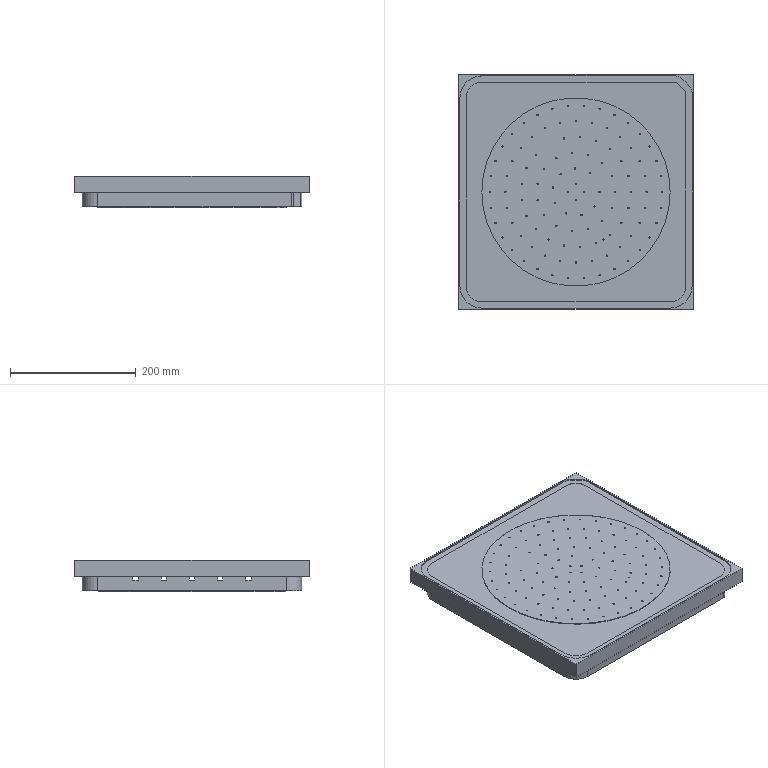NC program | NX | posted with a generic post | part box 374 x 374 x 49.5 mm
Lines 1180 to 2421 of 17720:
(03 , TOOL : D10)
N2352 M6
N2354 G53
N2356 G17 G0 G90 X-180. Y87.278 S7000 M3 M8
N2358 G43 Z105.5 H0
N2360 Z25.
N2362 G94 G1 Y125.441 Z23. F4000.
N2364 Y150.
N2366 G2 X-150. Y180. R30.
N2368 G1 X157.929
N2370 G2 X165. Y177.071 R10.
N2372 G1 X177.071 Y165.
N2374 G2 X180. Y157.929 R10.
N2376 G1 Y-150.
N2378 G2 X150. Y-180. R30.
N2380 G1 X-150.
N2382 G2 X-180. Y-150. R30.
N2384 G1 Y125.441
N2386 X-173.
N2388 Y150.
N2390 G2 X-150. Y173. R23.
N2392 G1 X157.929
N2394 G2 X160.05 Y172.121 R3.
N2396 G1 X172.121 Y160.05
N2398 G2 X173. Y157.929 R3.
N2400 G1 Y-150.
N2402 G2 X150. Y-173. R23.
N2404 G1 X-150.
N2406 G2 X-173. Y-150. R23.
N2408 G1 Y125.441
N2410 X-166.
N2412 Y150.
N2414 G2 X-150. Y166. R16.
N2416 G1 X156.272
N2418 X166. Y156.272
N2420 Y-150.
N2422 G2 X150. Y-166. R16.
N2424 G1 X-150.
N2426 G2 X-166. Y-150. R16.
N2428 G1 Y125.441
N2430 X-159.
N2432 Y150.
N2434 G2 X-150. Y159. R9.
N2436 G1 X153.373
N2438 X159. Y153.373
N2440 Y36.837
N2442 X152.
N2444 G3 X36.837 Y152. R156.4
N2446 G1 X30.515 Y153.705
N2448 X36.837 Y152.
N2450 X150.473
N2452 X152. Y150.473
N2454 Y75.33
N2456 X145.
N2458 G3 X75.33 Y145. R163.4
N2460 G1 X69.214 Y146.433
N2462 X75.33 Y145.
N2464 X145.
N2466 Y99.961
N2468 X138.
N2470 G3 X99.961 Y138. R170.4
N2472 G1 X94.665 Y139.672
N2474 X99.961 Y138.
N2476 X138.
N2478 Y119.623
N2480 X131.
N2482 G3 X119.623 Y131. R177.4
N2484 G1 X114.752 Y132.852
N2486 X119.623 Y131.
N2488 X131.
N2490 Y119.623
N2492 X132.852 Y114.752
N2494 X131. Y119.623
N2496 X138.
N2498 Y99.961
N2500 X139.672 Y94.665
N2502 X138. Y99.961
N2504 X145.
N2506 Y75.33
N2508 X146.433 Y69.214
N2510 X145. Y75.33
N2512 X152.
N2514 Y36.837
N2516 X153.705 Y30.515
N2518 X152. Y36.837
N2520 X159.
N2522 Y-150.
N2524 G2 X150. Y-159. R9.
N2526 G1 X36.837
N2528 Y-152.
N2530 G3 X152. Y-36.837 R156.4
N2532 G1 X153.705 Y-30.515
N2534 X152. Y-36.837
N2536 Y-150.
N2538 G2 X150. Y-152. R2.
N2540 G1 X75.33
N2542 Y-145.
N2544 G3 X145. Y-75.33 R163.4
N2546 G1 X146.433 Y-69.214
N2548 X145. Y-75.33
N2550 Y-145.
N2552 X99.961
N2554 Y-138.
N2556 G3 X138. Y-99.961 R170.4
N2558 G1 X139.672 Y-94.665
N2560 X138. Y-99.961
N2562 Y-138.
N2564 X119.623
N2566 Y-131.
N2568 G3 X131. Y-119.623 R177.4
N2570 G1 X132.852 Y-114.752
N2572 X131. Y-119.623
N2574 Y-131.
N2576 X119.623
N2578 X114.752 Y-132.852
N2580 X119.623 Y-131.
N2582 Y-138.
N2584 X99.961
N2586 X94.665 Y-139.672
N2588 X99.961 Y-138.
N2590 Y-145.
N2592 X75.33
N2594 X69.214 Y-146.433
N2596 X75.33 Y-145.
N2598 Y-152.
N2600 X36.837
N2602 X30.515 Y-153.705
N2604 X36.837 Y-152.
N2606 Y-159.
N2608 X-150.
N2610 G2 X-159. Y-150. R9.
N2612 G1 Y-36.837
N2614 X-152.
N2616 G3 X-36.837 Y-152. R156.4
N2618 G1 X-30.515 Y-153.705
N2620 X-36.837 Y-152.
N2622 X-150.
N2624 G2 X-152. Y-150. R2.
N2626 G1 Y-75.33
N2628 X-145.
N2630 G3 X-75.33 Y-145. R163.4
N2632 G1 X-69.214 Y-146.433
N2634 X-75.33 Y-145.
N2636 X-145.
N2638 Y-99.961
N2640 X-138.
N2642 G3 X-99.961 Y-138. R170.4
N2644 G1 X-94.665 Y-139.672
N2646 X-99.961 Y-138.
N2648 X-138.
N2650 Y-119.623
N2652 X-131.
N2654 G3 X-119.623 Y-131. R177.4
N2656 G1 X-114.752 Y-132.852
N2658 X-119.623 Y-131.
N2660 X-131.
N2662 Y-119.623
N2664 X-132.852 Y-114.752
N2666 X-131. Y-119.623
N2668 X-138.
N2670 Y-99.961
N2672 X-139.672 Y-94.665
N2674 X-138. Y-99.961
N2676 X-145.
N2678 Y-75.33
N2680 X-146.433 Y-69.214
N2682 X-145. Y-75.33
N2684 X-152.
N2686 Y-36.837
N2688 X-153.705 Y-30.515
N2690 X-152. Y-36.837
N2692 X-159.
N2694 Y125.441
N2696 X-152.
N2698 Y150.
N2700 G2 X-150. Y152. R2.
N2702 G1 X-36.837
N2704 X-30.515 Y153.705
N2706 X-36.837 Y152.
N2708 G3 X-152. Y36.837 R156.4
N2710 G1 X-153.705 Y30.515
N2712 X-152. Y36.837
N2714 X-150.639 Y36.507
N2716 G2 X36.507 Y150.639 R155.
N2718 X-150.639 Y36.507 R-155.
N2720 G1 X-152. Y36.837
N2722 Y125.441
N2724 X-145.
N2726 Y145.
N2728 X-75.33
N2730 X-69.214 Y146.433
N2732 X-75.33 Y145.
N2734 G3 X-145. Y75.33 R163.4
N2736 G1 X-146.433 Y69.214
N2738 X-145. Y75.33
N2740 Y125.441
N2742 X-138.
N2744 Y138.
N2746 X-99.961
N2748 X-94.665 Y139.672
N2750 X-99.961 Y138.
N2752 G3 X-138. Y99.961 R170.4
N2754 G1 X-139.672 Y94.665
N2756 X-138. Y99.961
N2758 Y125.441
N2760 X-131.
N2762 Y131.
N2764 X-119.623
N2766 X-114.752 Y132.852
N2768 X-119.623 Y131.
N2770 G3 X-131. Y119.623 R177.4
N2772 G1 X-132.852 Y114.752
N2774 X-131. Y119.623
N2776 Y125.441
N2778 G3 X-133. Y127.441 R2.
N2780 G1 Z24.
N2782 G0 Z105.5
N2784 X-148.274 Y-37.767
N2786 Z26.
N2788 G1 X-148.508 Y-36.927 Z25.954
N2790 X-150.341 Y-28.56 Z25.505
N2792 X-151.704 Y-20.104 Z25.057
N2794 X-152.591 Y-11.585 Z24.608
N2796 X-153. Y-3.03 Z24.159
N2798 Y0. Z24.
N2800 G2 X0. Y153. R153.
N2802 X-153. Y0. R-153.
N2804 G1 X-146.
N2806 G2 X0. Y146. R146.
N2808 X-146. Y0. R-146.
N2810 G1 X-139.
N2812 G2 X0. Y139. R139.
N2814 X-139. Y0. R-139.
N2816 G1 X-132.
N2818 G2 X0. Y132. R132.
N2820 X-132. Y0. R-132.
N2822 G1 X-125.
N2824 G2 X0. Y125. R125.
N2826 X-125. Y0. R-125.
N2828 G1 X-118.
N2830 G2 X0. Y118. R118.
N2832 X-118. Y0. R-118.
N2834 G1 X-111.
N2836 G2 X0. Y111. R111.
N2838 X-111. Y0. R-111.
N2840 G1 X-104.
N2842 G2 X0. Y104. R104.
N2844 X-104. Y0. R-104.
N2846 G1 X-97.
N2848 G2 X0. Y97. R97.
N2850 X-97. Y0. R-97.
N2852 G1 X-90.
N2854 G2 X0. Y90. R90.
N2856 X-90. Y0. R-90.
N2858 G1 X-83.
N2860 G2 X0. Y83. R83.
N2862 X-83. Y0. R-83.
N2864 G1 X-76.
N2866 G2 X0. Y76. R76.
N2868 X-76. Y0. R-76.
N2870 G1 X-69.
N2872 G2 X0. Y69. R69.
N2874 X-69. Y0. R-69.
N2876 G1 X-62.
N2878 G2 X0. Y62. R62.
N2880 X-62. Y0. R-62.
N2882 G1 X-55.
N2884 G2 X0. Y55. R55.
N2886 X-55. Y0. R-55.
N2888 G1 X-48.
N2890 G2 X0. Y48. R48.
N2892 X-48. Y0. R-48.
N2894 G1 X-41.
N2896 G2 X0. Y41. R41.
N2898 X-41. Y0. R-41.
N2900 G1 X-34.
N2902 G2 X0. Y34. R34.
N2904 X-34. Y0. R-34.
N2906 G1 X-27.
N2908 G2 X0. Y27. R27.
N2910 X-27. Y0. R-27.
N2912 G1 X-20.
N2914 G2 X0. Y20. R20.
N2916 X-20. Y0. R-20.
N2918 G1 X-13.
N2920 G2 X0. Y13. R13.
N2922 X-13. Y0. R-13.
N2924 G1 X-6.
N2926 G2 X0. Y6. R6.
N2928 X-6. Y0. R-6.
N2930 G1 X-1.5
N2932 G2 X0. Y1.5 R1.5
N2934 X-1.5 Y0. R-1.5
N2936 G3 X-3.5 Y2. R2.
N2938 G1 Z25.
N2940 G0 Z105.5
(003 , TOOL : D10)
N2942 X176.276 Y165.795
N2944 Z24.
N2946 G1 X177.619 Y164.452 Z23.998
N2948 X178.813 Y162.718 Z23.997
N2950 X179.618 Y160.774 Z23.995
N2952 X180. Y158.704 Z23.993
N2954 Y-151.342 Z23.722
N2956 X179.606 Y-155.026 Z23.719
N2958 X178.762 Y-158.633 Z23.716
N2960 X177.48 Y-162.109 Z23.713
N2962 X175.78 Y-165.401 Z23.709
N2964 X173.688 Y-168.458 Z23.706
N2966 X171.234 Y-171.234 Z23.703
N2968 X168.458 Y-173.688 Z23.7
N2970 X165.401 Y-175.78 Z23.696
N2972 X162.109 Y-177.48 Z23.693
N2974 X158.633 Y-178.762 Z23.69
N2976 X155.026 Y-179.606 Z23.687
N2978 X151.342 Y-180. Z23.683
N2980 X-151.342 Z23.419
N2982 X-155.026 Y-179.606 Z23.416
N2984 X-158.633 Y-178.762 Z23.413
N2986 X-162.109 Y-177.48 Z23.41
N2988 X-165.401 Y-175.78 Z23.406
N2990 X-168.458 Y-173.688 Z23.403
N2992 X-171.234 Y-171.234 Z23.4
N2994 X-173.688 Y-168.458 Z23.397
N2996 X-175.78 Y-165.401 Z23.393
N2998 X-177.48 Y-162.109 Z23.39
N3000 X-178.762 Y-158.633 Z23.387
N3002 X-179.606 Y-155.026 Z23.384
N3004 X-180. Y-151.342 Z23.381
N3006 Y151.342 Z23.116
N3008 X-179.606 Y155.026 Z23.113
N3010 X-178.762 Y158.633 Z23.11
N3012 X-177.48 Y162.109 Z23.107
N3014 X-175.78 Y165.401 Z23.103
N3016 X-173.688 Y168.458 Z23.1
N3018 X-171.234 Y171.234 Z23.097
N3020 X-168.458 Y173.688 Z23.094
N3022 X-165.401 Y175.78 Z23.091
N3024 X-162.109 Y177.48 Z23.087
N3026 X-158.633 Y178.762 Z23.084
N3028 X-155.026 Y179.606 Z23.081
N3030 X-151.342 Y180. Z23.078
N3032 X158.704 Z22.807
N3034 X160.774 Y179.618 Z22.805
N3036 X162.718 Y178.813 Z22.803
N3038 X164.452 Y177.619 Z22.802
N3040 X177.619 Y164.452 Z22.785
N3042 X178.813 Y162.718 Z22.783
N3044 X179.618 Y160.774 Z22.782
N3046 X180. Y158.704 Z22.78
N3048 Y-151.342 Z22.509
N3050 X179.606 Y-155.026 Z22.506
N3052 X178.762 Y-158.633 Z22.503
N3054 X177.48 Y-162.109 Z22.499
N3056 X175.78 Y-165.401 Z22.496
N3058 X173.688 Y-168.458 Z22.493
N3060 X171.234 Y-171.234 Z22.49
N3062 X168.458 Y-173.688 Z22.487
N3064 X165.401 Y-175.78 Z22.483
N3066 X162.109 Y-177.48 Z22.48
N3068 X158.633 Y-178.762 Z22.477
N3070 X155.026 Y-179.606 Z22.474
N3072 X151.342 Y-180. Z22.47
N3074 X-151.342 Z22.206
N3076 X-155.026 Y-179.606 Z22.203
N3078 X-158.633 Y-178.762 Z22.2
N3080 X-162.109 Y-177.48 Z22.197
N3082 X-165.401 Y-175.78 Z22.193
N3084 X-168.458 Y-173.688 Z22.19
N3086 X-171.234 Y-171.234 Z22.187
N3088 X-173.688 Y-168.458 Z22.184
N3090 X-175.78 Y-165.401 Z22.18
N3092 X-177.48 Y-162.109 Z22.177
N3094 X-178.762 Y-158.633 Z22.174
N3096 X-179.606 Y-155.026 Z22.171
N3098 X-180. Y-151.342 Z22.167
N3100 Y151.342 Z21.903
N3102 X-179.606 Y155.026 Z21.9
N3104 X-178.762 Y158.633 Z21.897
N3106 X-177.48 Y162.109 Z21.894
N3108 X-175.78 Y165.401 Z21.89
N3110 X-173.688 Y168.458 Z21.887
N3112 X-171.234 Y171.234 Z21.884
N3114 X-168.458 Y173.688 Z21.881
N3116 X-165.401 Y175.78 Z21.877
N3118 X-162.109 Y177.48 Z21.874
N3120 X-158.633 Y178.762 Z21.871
N3122 X-155.026 Y179.606 Z21.868
N3124 X-151.342 Y180. Z21.865
N3126 X158.704 Z21.594
N3128 X160.774 Y179.618 Z21.592
N3130 X162.718 Y178.813 Z21.59
N3132 X164.452 Y177.619 Z21.588
N3134 X177.619 Y164.452 Z21.572
N3136 X178.813 Y162.718 Z21.57
N3138 X179.618 Y160.774 Z21.569
N3140 X180. Y158.704 Z21.567
N3142 Y-151.342 Z21.296
N3144 X179.606 Y-155.026 Z21.293
N3146 X178.762 Y-158.633 Z21.29
N3148 X177.48 Y-162.109 Z21.286
N3150 X175.78 Y-165.401 Z21.283
N3152 X173.688 Y-168.458 Z21.28
N3154 X171.234 Y-171.234 Z21.277
N3156 X168.458 Y-173.688 Z21.273
N3158 X165.401 Y-175.78 Z21.27
N3160 X162.109 Y-177.48 Z21.267
N3162 X158.633 Y-178.762 Z21.264
N3164 X155.026 Y-179.606 Z21.261
N3166 X151.342 Y-180. Z21.257
N3168 X-151.342 Z20.993
N3170 X-155.026 Y-179.606 Z20.99
N3172 X-158.633 Y-178.762 Z20.987
N3174 X-162.109 Y-177.48 Z20.983
N3176 X-165.401 Y-175.78 Z20.98
N3178 X-168.458 Y-173.688 Z20.977
N3180 X-171.234 Y-171.234 Z20.974
N3182 X-173.688 Y-168.458 Z20.971
N3184 X-175.78 Y-165.401 Z20.967
N3186 X-177.48 Y-162.109 Z20.964
N3188 X-178.762 Y-158.633 Z20.961
N3190 X-179.606 Y-155.026 Z20.958
N3192 X-180. Y-151.342 Z20.954
N3194 Y151.342 Z20.69
N3196 X-179.606 Y155.026 Z20.687
N3198 X-178.762 Y158.633 Z20.684
N3200 X-177.48 Y162.109 Z20.681
N3202 X-175.78 Y165.401 Z20.677
N3204 X-173.688 Y168.458 Z20.674
N3206 X-171.234 Y171.234 Z20.671
N3208 X-168.458 Y173.688 Z20.668
N3210 X-165.401 Y175.78 Z20.664
N3212 X-162.109 Y177.48 Z20.661
N3214 X-158.633 Y178.762 Z20.658
N3216 X-155.026 Y179.606 Z20.655
N3218 X-151.342 Y180. Z20.651
N3220 X158.704 Z20.381
N3222 X160.774 Y179.618 Z20.379
N3224 X162.718 Y178.813 Z20.377
N3226 X164.452 Y177.619 Z20.375
N3228 X177.619 Y164.452 Z20.359
N3230 X178.813 Y162.718 Z20.357
N3232 X179.618 Y160.774 Z20.355
N3234 X180. Y158.704 Z20.354
N3236 Y-151.342 Z20.083
N3238 X179.606 Y-155.026 Z20.08
N3240 X178.762 Y-158.633 Z20.077
N3242 X177.48 Y-162.109 Z20.073
N3244 X175.78 Y-165.401 Z20.07
N3246 X173.688 Y-168.458 Z20.067
N3248 X171.234 Y-171.234 Z20.064
N3250 X168.458 Y-173.688 Z20.06
N3252 X165.401 Y-175.78 Z20.057
N3254 X162.109 Y-177.48 Z20.054
N3256 X158.633 Y-178.762 Z20.051
N3258 X155.026 Y-179.606 Z20.047
N3260 X151.342 Y-180. Z20.044
N3262 X-151.342 Z19.78
N3264 X-155.026 Y-179.606 Z19.777
N3266 X-158.633 Y-178.762 Z19.774
N3268 X-162.109 Y-177.48 Z19.77
N3270 X-165.401 Y-175.78 Z19.767
N3272 X-168.458 Y-173.688 Z19.764
N3274 X-171.234 Y-171.234 Z19.761
N3276 X-173.688 Y-168.458 Z19.757
N3278 X-175.78 Y-165.401 Z19.754
N3280 X-177.48 Y-162.109 Z19.751
N3282 X-178.762 Y-158.633 Z19.748
N3284 X-179.606 Y-155.026 Z19.745
N3286 X-180. Y-151.342 Z19.741
N3288 Y151.342 Z19.477
N3290 X-179.606 Y155.026 Z19.474
N3292 X-178.762 Y158.633 Z19.471
N3294 X-177.48 Y162.109 Z19.467
N3296 X-175.78 Y165.401 Z19.464
N3298 X-173.688 Y168.458 Z19.461
N3300 X-171.234 Y171.234 Z19.458
N3302 X-168.458 Y173.688 Z19.455
N3304 X-165.401 Y175.78 Z19.451
N3306 X-162.109 Y177.48 Z19.448
N3308 X-158.633 Y178.762 Z19.445
N3310 X-155.026 Y179.606 Z19.442
N3312 X-151.342 Y180. Z19.438
N3314 X158.704 Z19.168
N3316 X160.774 Y179.618 Z19.166
N3318 X162.718 Y178.813 Z19.164
N3320 X164.452 Y177.619 Z19.162
N3322 X177.619 Y164.452 Z19.146
N3324 X178.813 Y162.718 Z19.144
N3326 X179.618 Y160.774 Z19.142
N3328 X180. Y158.704 Z19.141
N3330 Y-151.342 Z18.87
N3332 X179.606 Y-155.026 Z18.867
N3334 X178.762 Y-158.633 Z18.863
N3336 X177.48 Y-162.109 Z18.86
N3338 X175.78 Y-165.401 Z18.857
N3340 X173.688 Y-168.458 Z18.854
N3342 X171.234 Y-171.234 Z18.851
N3344 X168.458 Y-173.688 Z18.847
N3346 X165.401 Y-175.78 Z18.844
N3348 X162.109 Y-177.48 Z18.841
N3350 X158.633 Y-178.762 Z18.838
N3352 X155.026 Y-179.606 Z18.834
N3354 X151.342 Y-180. Z18.831
N3356 X-151.342 Z18.567
N3358 X-155.026 Y-179.606 Z18.564
N3360 X-158.633 Y-178.762 Z18.561
N3362 X-162.109 Y-177.48 Z18.557
N3364 X-165.401 Y-175.78 Z18.554
N3366 X-168.458 Y-173.688 Z18.551
N3368 X-171.234 Y-171.234 Z18.548
N3370 X-173.688 Y-168.458 Z18.544
N3372 X-175.78 Y-165.401 Z18.541
N3374 X-177.48 Y-162.109 Z18.538
N3376 X-178.762 Y-158.633 Z18.535
N3378 X-179.606 Y-155.026 Z18.531
N3380 X-180. Y-151.342 Z18.528
N3382 Y151.342 Z18.264
N3384 X-179.606 Y155.026 Z18.261
N3386 X-178.762 Y158.633 Z18.258
N3388 X-177.48 Y162.109 Z18.254
N3390 X-175.78 Y165.401 Z18.251
N3392 X-173.688 Y168.458 Z18.248
N3394 X-171.234 Y171.234 Z18.245
N3396 X-168.458 Y173.688 Z18.241
N3398 X-165.401 Y175.78 Z18.238
N3400 X-162.109 Y177.48 Z18.235
N3402 X-158.633 Y178.762 Z18.232
N3404 X-155.026 Y179.606 Z18.229
N3406 X-151.342 Y180. Z18.225
N3408 X158.704 Z17.955
N3410 X160.774 Y179.618 Z17.953
N3412 X162.718 Y178.813 Z17.951
N3414 X164.452 Y177.619 Z17.949
N3416 X177.619 Y164.452 Z17.933
N3418 X178.813 Y162.718 Z17.931
N3420 X179.618 Y160.774 Z17.929
N3422 X180. Y158.704 Z17.927
N3424 Y-151.342 Z17.657
N3426 X179.606 Y-155.026 Z17.654
N3428 X178.762 Y-158.633 Z17.65
N3430 X177.48 Y-162.109 Z17.647
N3432 X175.78 Y-165.401 Z17.644
N3434 X173.688 Y-168.458 Z17.641
N3436 X171.234 Y-171.234 Z17.637
N3438 X168.458 Y-173.688 Z17.634
N3440 X165.401 Y-175.78 Z17.631
N3442 X162.109 Y-177.48 Z17.628
N3444 X158.633 Y-178.762 Z17.625
N3446 X155.026 Y-179.606 Z17.621
N3448 X151.342 Y-180. Z17.618
N3450 X-151.342 Z17.354
N3452 X-155.026 Y-179.606 Z17.351
N3454 X-158.633 Y-178.762 Z17.347
N3456 X-162.109 Y-177.48 Z17.344
N3458 X-165.401 Y-175.78 Z17.341
N3460 X-168.458 Y-173.688 Z17.338
N3462 X-171.234 Y-171.234 Z17.335
N3464 X-173.688 Y-168.458 Z17.331
N3466 X-175.78 Y-165.401 Z17.328
N3468 X-177.48 Y-162.109 Z17.325
N3470 X-178.762 Y-158.633 Z17.322
N3472 X-179.606 Y-155.026 Z17.318
N3474 X-180. Y-151.342 Z17.315
N3476 Y151.342 Z17.051
N3478 X-179.606 Y155.026 Z17.048
N3480 X-178.762 Y158.633 Z17.045
N3482 X-177.48 Y162.109 Z17.041
N3484 X-175.78 Y165.401 Z17.038
N3486 X-173.688 Y168.458 Z17.035
N3488 X-171.234 Y171.234 Z17.032
N3490 X-168.458 Y173.688 Z17.028
N3492 X-165.401 Y175.78 Z17.025
N3494 X-162.109 Y177.48 Z17.022
N3496 X-158.633 Y178.762 Z17.019
N3498 X-155.026 Y179.606 Z17.015
N3500 X-151.342 Y180. Z17.012
N3502 X158.704 Z16.742
N3504 X160.774 Y179.618 Z16.74
N3506 X162.718 Y178.813 Z16.738
N3508 X164.452 Y177.619 Z16.736
N3510 X177.619 Y164.452 Z16.72
N3512 X178.813 Y162.718 Z16.718
N3514 X179.618 Y160.774 Z16.716
N3516 X180. Y158.704 Z16.714
N3518 Y-151.342 Z16.444
N3520 X179.606 Y-155.026 Z16.441
N3522 X178.762 Y-158.633 Z16.437
N3524 X177.48 Y-162.109 Z16.434
N3526 X175.78 Y-165.401 Z16.431
N3528 X173.688 Y-168.458 Z16.428
N3530 X171.234 Y-171.234 Z16.424
N3532 X168.458 Y-173.688 Z16.421
N3534 X165.401 Y-175.78 Z16.418
N3536 X162.109 Y-177.48 Z16.415
N3538 X158.633 Y-178.762 Z16.411
N3540 X155.026 Y-179.606 Z16.408
N3542 X151.342 Y-180. Z16.405
N3544 X-151.342 Z16.141
N3546 X-155.026 Y-179.606 Z16.138
N3548 X-158.633 Y-178.762 Z16.134
N3550 X-162.109 Y-177.48 Z16.131
N3552 X-165.401 Y-175.78 Z16.128
N3554 X-168.458 Y-173.688 Z16.125
N3556 X-171.234 Y-171.234 Z16.121
N3558 X-173.688 Y-168.458 Z16.118
N3560 X-175.78 Y-165.401 Z16.115
N3562 X-177.48 Y-162.109 Z16.112
N3564 X-178.762 Y-158.633 Z16.109
N3566 X-179.606 Y-155.026 Z16.105
N3568 X-180. Y-151.342 Z16.102
N3570 Y151.342 Z15.838
N3572 X-179.606 Y155.026 Z15.835
N3574 X-178.762 Y158.633 Z15.831
N3576 X-177.48 Y162.109 Z15.828
N3578 X-175.78 Y165.401 Z15.825
N3580 X-173.688 Y168.458 Z15.822
N3582 X-171.234 Y171.234 Z15.819
N3584 X-168.458 Y173.688 Z15.815
N3586 X-165.401 Y175.78 Z15.812
N3588 X-162.109 Y177.48 Z15.809
N3590 X-158.633 Y178.762 Z15.806
N3592 X-155.026 Y179.606 Z15.802
N3594 X-151.342 Y180. Z15.799
N3596 X158.704 Z15.529
N3598 X160.774 Y179.618 Z15.527
N3600 X162.718 Y178.813 Z15.525
N3602 X164.452 Y177.619 Z15.523
N3604 X177.619 Y164.452 Z15.507
N3606 X178.813 Y162.718 Z15.505
N3608 X179.618 Y160.774 Z15.503
N3610 X180. Y158.704 Z15.501
N3612 Y-151.342 Z15.231
N3614 X179.606 Y-155.026 Z15.227
N3616 X178.762 Y-158.633 Z15.224
N3618 X177.48 Y-162.109 Z15.221
N3620 X175.78 Y-165.401 Z15.218
N3622 X173.688 Y-168.458 Z15.215
N3624 X171.234 Y-171.234 Z15.211
N3626 X168.458 Y-173.688 Z15.208
N3628 X165.401 Y-175.78 Z15.205
N3630 X162.109 Y-177.48 Z15.202
N3632 X158.633 Y-178.762 Z15.198
N3634 X155.026 Y-179.606 Z15.195
N3636 X151.342 Y-180. Z15.192
N3638 X-151.342 Z14.928
N3640 X-155.026 Y-179.606 Z14.925
N3642 X-158.633 Y-178.762 Z14.921
N3644 X-162.109 Y-177.48 Z14.918
N3646 X-165.401 Y-175.78 Z14.915
N3648 X-168.458 Y-173.688 Z14.912
N3650 X-171.234 Y-171.234 Z14.908
N3652 X-173.688 Y-168.458 Z14.905
N3654 X-175.78 Y-165.401 Z14.902
N3656 X-177.48 Y-162.109 Z14.899
N3658 X-178.762 Y-158.633 Z14.895
N3660 X-179.606 Y-155.026 Z14.892
N3662 X-180. Y-151.342 Z14.889
N3664 Y151.342 Z14.625
N3666 X-179.606 Y155.026 Z14.622
N3668 X-178.762 Y158.633 Z14.618
N3670 X-177.48 Y162.109 Z14.615
N3672 X-175.78 Y165.401 Z14.612
N3674 X-173.688 Y168.458 Z14.609
N3676 X-171.234 Y171.234 Z14.605
N3678 X-168.458 Y173.688 Z14.602
N3680 X-165.401 Y175.78 Z14.599
N3682 X-162.109 Y177.48 Z14.596
N3684 X-158.633 Y178.762 Z14.593
N3686 X-155.026 Y179.606 Z14.589
N3688 X-151.342 Y180. Z14.586
N3690 X158.704 Z14.315
N3692 X160.774 Y179.618 Z14.314
N3694 X162.718 Y178.813 Z14.312
N3696 X164.452 Y177.619 Z14.31
N3698 X177.619 Y164.452 Z14.294
N3700 X178.813 Y162.718 Z14.292
N3702 X179.618 Y160.774 Z14.29
N3704 X180. Y158.704 Z14.288
N3706 Y-151.342 Z14.018
N3708 X179.606 Y-155.026 Z14.014
N3710 X178.762 Y-158.633 Z14.011
N3712 X177.48 Y-162.109 Z14.008
N3714 X175.78 Y-165.401 Z14.005
N3716 X173.688 Y-168.458 Z14.001
N3718 X171.234 Y-171.234 Z13.998
N3720 X168.458 Y-173.688 Z13.995
N3722 X165.401 Y-175.78 Z13.992
N3724 X162.109 Y-177.48 Z13.989
N3726 X158.633 Y-178.762 Z13.985
N3728 X155.026 Y-179.606 Z13.982
N3730 X151.342 Y-180. Z13.979
N3732 X-151.342 Z13.715
N3734 X-155.026 Y-179.606 Z13.711
N3736 X-158.633 Y-178.762 Z13.708
N3738 X-162.109 Y-177.48 Z13.705
N3740 X-165.401 Y-175.78 Z13.702
N3742 X-168.458 Y-173.688 Z13.699
N3744 X-171.234 Y-171.234 Z13.695
N3746 X-173.688 Y-168.458 Z13.692
N3748 X-175.78 Y-165.401 Z13.689
N3750 X-177.48 Y-162.109 Z13.686
N3752 X-178.762 Y-158.633 Z13.682
N3754 X-179.606 Y-155.026 Z13.679
N3756 X-180. Y-151.342 Z13.676
N3758 Y151.342 Z13.412
N3760 X-179.606 Y155.026 Z13.409
N3762 X-178.762 Y158.633 Z13.405
N3764 X-177.48 Y162.109 Z13.402
N3766 X-175.78 Y165.401 Z13.399
N3768 X-173.688 Y168.458 Z13.396
N3770 X-171.234 Y171.234 Z13.392
N3772 X-168.458 Y173.688 Z13.389
N3774 X-165.401 Y175.78 Z13.386
N3776 X-162.109 Y177.48 Z13.383
N3778 X-158.633 Y178.762 Z13.379
N3780 X-155.026 Y179.606 Z13.376
N3782 X-151.342 Y180. Z13.373
N3784 X158.704 Z13.102
N3786 X160.774 Y179.618 Z13.101
N3788 X162.718 Y178.813 Z13.099
N3790 X164.452 Y177.619 Z13.097
N3792 X177.619 Y164.452 Z13.081
N3794 X178.813 Y162.718 Z13.079
N3796 X179.618 Y160.774 Z13.077
N3798 X180. Y158.704 Z13.075
N3800 Y-151.342 Z12.805
N3802 X179.606 Y-155.026 Z12.801
N3804 X178.762 Y-158.633 Z12.798
N3806 X177.48 Y-162.109 Z12.795
N3808 X175.78 Y-165.401 Z12.792
N3810 X173.688 Y-168.458 Z12.788
N3812 X171.234 Y-171.234 Z12.785
N3814 X168.458 Y-173.688 Z12.782
N3816 X165.401 Y-175.78 Z12.779
N3818 X162.109 Y-177.48 Z12.775
N3820 X158.633 Y-178.762 Z12.772
N3822 X155.026 Y-179.606 Z12.769
N3824 X151.342 Y-180. Z12.766
N3826 X-151.342 Z12.502
N3828 X-155.026 Y-179.606 Z12.498
N3830 X-158.633 Y-178.762 Z12.495
N3832 X-162.109 Y-177.48 Z12.492
N3834 X-165.401 Y-175.78 Z12.489
N3836 X-168.458 Y-173.688 Z12.485
N3838 X-171.234 Y-171.234 Z12.482
N3840 X-173.688 Y-168.458 Z12.479
N3842 X-175.78 Y-165.401 Z12.476
N3844 X-177.48 Y-162.109 Z12.473
N3846 X-178.762 Y-158.633 Z12.469
N3848 X-179.606 Y-155.026 Z12.466
N3850 X-180. Y-151.342 Z12.463
N3852 Y151.342 Z12.199
N3854 X-179.606 Y155.026 Z12.195
N3856 X-178.762 Y158.633 Z12.192
N3858 X-177.48 Y162.109 Z12.189
N3860 X-175.78 Y165.401 Z12.186
N3862 X-173.688 Y168.458 Z12.183
N3864 X-171.234 Y171.234 Z12.179
N3866 X-168.458 Y173.688 Z12.176
N3868 X-165.401 Y175.78 Z12.173
N3870 X-162.109 Y177.48 Z12.17
N3872 X-158.633 Y178.762 Z12.166
N3874 X-155.026 Y179.606 Z12.163
N3876 X-151.342 Y180. Z12.16
N3878 X158.704 Z11.889
N3880 X160.774 Y179.618 Z11.887
N3882 X162.718 Y178.813 Z11.886
N3884 X164.452 Y177.619 Z11.884
N3886 X177.619 Y164.452 Z11.868
N3888 X178.813 Y162.718 Z11.866
N3890 X179.618 Y160.774 Z11.864
N3892 X180. Y158.704 Z11.862
N3894 Y-151.342 Z11.591
N3896 X179.606 Y-155.026 Z11.588
N3898 X178.762 Y-158.633 Z11.585
N3900 X177.48 Y-162.109 Z11.582
N3902 X175.78 Y-165.401 Z11.579
N3904 X173.688 Y-168.458 Z11.575
N3906 X171.234 Y-171.234 Z11.572
N3908 X168.458 Y-173.688 Z11.569
N3910 X165.401 Y-175.78 Z11.566
N3912 X162.109 Y-177.48 Z11.562
N3914 X158.633 Y-178.762 Z11.559
N3916 X155.026 Y-179.606 Z11.556
N3918 X151.342 Y-180. Z11.553
N3920 X-151.342 Z11.289
N3922 X-155.026 Y-179.606 Z11.285
N3924 X-158.633 Y-178.762 Z11.282
N3926 X-162.109 Y-177.48 Z11.279
N3928 X-165.401 Y-175.78 Z11.276
N3930 X-168.458 Y-173.688 Z11.272
N3932 X-171.234 Y-171.234 Z11.269
N3934 X-173.688 Y-168.458 Z11.266
N3936 X-175.78 Y-165.401 Z11.263
N3938 X-177.48 Y-162.109 Z11.259
N3940 X-178.762 Y-158.633 Z11.256
N3942 X-179.606 Y-155.026 Z11.253
N3944 X-180. Y-151.342 Z11.25
N3946 Y151.342 Z10.986
N3948 X-179.606 Y155.026 Z10.982
N3950 X-178.762 Y158.633 Z10.979
N3952 X-177.48 Y162.109 Z10.976
N3954 X-175.78 Y165.401 Z10.973
N3956 X-173.688 Y168.458 Z10.969
N3958 X-171.234 Y171.234 Z10.966
N3960 X-168.458 Y173.688 Z10.963
N3962 X-165.401 Y175.78 Z10.96
N3964 X-162.109 Y177.48 Z10.957
N3966 X-158.633 Y178.762 Z10.953
N3968 X-155.026 Y179.606 Z10.95
N3970 X-151.342 Y180. Z10.947
N3972 X158.704 Z10.676
N3974 X160.774 Y179.618 Z10.674
N3976 X162.718 Y178.813 Z10.673
N3978 X164.452 Y177.619 Z10.671
N3980 X177.619 Y164.452 Z10.654
N3982 X178.813 Y162.718 Z10.653
N3984 X179.618 Y160.774 Z10.651
N3986 X180. Y158.704 Z10.649
N3988 Y-151.342 Z10.378
N3990 X179.606 Y-155.026 Z10.375
N3992 X178.762 Y-158.633 Z10.372
N3994 X177.48 Y-162.109 Z10.369
N3996 X175.78 Y-165.401 Z10.365
N3998 X173.688 Y-168.458 Z10.362
N4000 X171.234 Y-171.234 Z10.359
N4002 X168.458 Y-173.688 Z10.356
N4004 X165.401 Y-175.78 Z10.353
N4006 X162.109 Y-177.48 Z10.349
N4008 X158.633 Y-178.762 Z10.346
N4010 X155.026 Y-179.606 Z10.343
N4012 X151.342 Y-180. Z10.34
N4014 X-151.342 Z10.075
N4016 X-155.026 Y-179.606 Z10.072
N4018 X-158.633 Y-178.762 Z10.069
N4020 X-162.109 Y-177.48 Z10.066
N4022 X-165.401 Y-175.78 Z10.063
N4024 X-168.458 Y-173.688 Z10.059
N4026 X-171.234 Y-171.234 Z10.056
N4028 X-173.688 Y-168.458 Z10.053
N4030 X-175.78 Y-165.401 Z10.05
N4032 X-177.48 Y-162.109 Z10.046
N4034 X-178.762 Y-158.633 Z10.043
N4036 X-179.606 Y-155.026 Z10.04
N4038 X-180. Y-151.342 Z10.037
N4040 Y151.342 Z9.773
N4042 X-179.606 Y155.026 Z9.769
N4044 X-178.762 Y158.633 Z9.766
N4046 X-177.48 Y162.109 Z9.763
N4048 X-175.78 Y165.401 Z9.76
N4050 X-173.688 Y168.458 Z9.756
N4052 X-171.234 Y171.234 Z9.753
N4054 X-168.458 Y173.688 Z9.75
N4056 X-165.401 Y175.78 Z9.747
N4058 X-162.109 Y177.48 Z9.743
N4060 X-158.633 Y178.762 Z9.74
N4062 X-155.026 Y179.606 Z9.737
N4064 X-151.342 Y180. Z9.734
N4066 X158.704 Z9.463
N4068 X160.774 Y179.618 Z9.461
N4070 X162.718 Y178.813 Z9.46
N4072 X164.452 Y177.619 Z9.458
N4074 X177.619 Y164.452 Z9.441
N4076 X178.813 Y162.718 Z9.44
N4078 X179.618 Y160.774 Z9.438
N4080 X180. Y158.704 Z9.436
N4082 Y-151.342 Z9.165
N4084 X179.606 Y-155.026 Z9.162
N4086 X178.762 Y-158.633 Z9.159
N4088 X177.48 Y-162.109 Z9.156
N4090 X175.78 Y-165.401 Z9.152
N4092 X173.688 Y-168.458 Z9.149
N4094 X171.234 Y-171.234 Z9.146
N4096 X168.458 Y-173.688 Z9.143
N4098 X165.401 Y-175.78 Z9.139
N4100 X162.109 Y-177.48 Z9.136
N4102 X158.633 Y-178.762 Z9.133
N4104 X155.026 Y-179.606 Z9.13
N4106 X151.342 Y-180. Z9.127
N4108 X-151.342 Z8.862
N4110 X-155.026 Y-179.606 Z8.859
N4112 X-158.633 Y-178.762 Z8.856
N4114 X-162.109 Y-177.48 Z8.853
N4116 X-165.401 Y-175.78 Z8.849
N4118 X-168.458 Y-173.688 Z8.846
N4120 X-171.234 Y-171.234 Z8.843
N4122 X-173.688 Y-168.458 Z8.84
N4124 X-175.78 Y-165.401 Z8.837
N4126 X-177.48 Y-162.109 Z8.833
N4128 X-178.762 Y-158.633 Z8.83
N4130 X-179.606 Y-155.026 Z8.827
N4132 X-180. Y-151.342 Z8.824
N4134 Y151.342 Z8.559
N4136 X-179.606 Y155.026 Z8.556
N4138 X-178.762 Y158.633 Z8.553
N4140 X-177.48 Y162.109 Z8.55
N4142 X-175.78 Y165.401 Z8.547
N4144 X-173.688 Y168.458 Z8.543
N4146 X-171.234 Y171.234 Z8.54
N4148 X-168.458 Y173.688 Z8.537
N4150 X-165.401 Y175.78 Z8.534
N4152 X-162.109 Y177.48 Z8.53
N4154 X-158.633 Y178.762 Z8.527
N4156 X-155.026 Y179.606 Z8.524
N4158 X-151.342 Y180. Z8.521
N4160 X158.704 Z8.25
N4162 X160.774 Y179.618 Z8.248
N4164 X162.718 Y178.813 Z8.246
N4166 X164.452 Y177.619 Z8.245
N4168 X177.619 Y164.452 Z8.228
N4170 X178.813 Y162.718 Z8.227
N4172 X179.618 Y160.774 Z8.225
N4174 X180. Y158.704 Z8.223
N4176 Y-151.342 Z7.952
N4178 X179.606 Y-155.026 Z7.949
N4180 X178.762 Y-158.633 Z7.946
N4182 X177.48 Y-162.109 Z7.943
N4184 X175.78 Y-165.401 Z7.939
N4186 X173.688 Y-168.458 Z7.936
N4188 X171.234 Y-171.234 Z7.933
N4190 X168.458 Y-173.688 Z7.93
N4192 X165.401 Y-175.78 Z7.926
N4194 X162.109 Y-177.48 Z7.923
N4196 X158.633 Y-178.762 Z7.92
N4198 X155.026 Y-179.606 Z7.917
N4200 X151.342 Y-180. Z7.913
N4202 X-151.342 Z7.649
N4204 X-155.026 Y-179.606 Z7.646
N4206 X-158.633 Y-178.762 Z7.643
N4208 X-162.109 Y-177.48 Z7.64
N4210 X-165.401 Y-175.78 Z7.636
N4212 X-168.458 Y-173.688 Z7.633
N4214 X-171.234 Y-171.234 Z7.63
N4216 X-173.688 Y-168.458 Z7.627
N4218 X-175.78 Y-165.401 Z7.623
N4220 X-177.48 Y-162.109 Z7.62
N4222 X-178.762 Y-158.633 Z7.617
N4224 X-179.606 Y-155.026 Z7.614
N4226 X-180. Y-151.342 Z7.611
N4228 Y151.342 Z7.346
N4230 X-179.606 Y155.026 Z7.343
N4232 X-178.762 Y158.633 Z7.34
N4234 X-177.48 Y162.109 Z7.337
N4236 X-175.78 Y165.401 Z7.333
N4238 X-173.688 Y168.458 Z7.33
N4240 X-171.234 Y171.234 Z7.327
N4242 X-168.458 Y173.688 Z7.324
N4244 X-165.401 Y175.78 Z7.321
N4246 X-162.109 Y177.48 Z7.317
N4248 X-158.633 Y178.762 Z7.314
N4250 X-155.026 Y179.606 Z7.311
N4252 X-151.342 Y180. Z7.308
N4254 X158.704 Z7.037
N4256 X160.774 Y179.618 Z7.035
N4258 X162.718 Y178.813 Z7.033
N4260 X164.452 Y177.619 Z7.032
N4262 X177.619 Y164.452 Z7.015
N4264 X178.813 Y162.718 Z7.013
N4266 X179.618 Y160.774 Z7.012
N4268 X180. Y158.704 Z7.01
N4270 Y-151.342 Z6.739
N4272 X179.606 Y-155.026 Z6.736
N4274 X178.762 Y-158.633 Z6.733
N4276 X177.48 Y-162.109 Z6.729
N4278 X175.78 Y-165.401 Z6.726
N4280 X173.688 Y-168.458 Z6.723
N4282 X171.234 Y-171.234 Z6.72
N4284 X168.458 Y-173.688 Z6.717
N4286 X165.401 Y-175.78 Z6.713
N4288 X162.109 Y-177.48 Z6.71
N4290 X158.633 Y-178.762 Z6.707
N4292 X155.026 Y-179.606 Z6.704
N4294 X151.342 Y-180. Z6.7
N4296 X-151.342 Z6.436
N4298 X-155.026 Y-179.606 Z6.433
N4300 X-158.633 Y-178.762 Z6.43
N4302 X-162.109 Y-177.48 Z6.427
N4304 X-165.401 Y-175.78 Z6.423
N4306 X-168.458 Y-173.688 Z6.42
N4308 X-171.234 Y-171.234 Z6.417
N4310 X-173.688 Y-168.458 Z6.414
N4312 X-175.78 Y-165.401 Z6.41
N4314 X-177.48 Y-162.109 Z6.407
N4316 X-178.762 Y-158.633 Z6.404
N4318 X-179.606 Y-155.026 Z6.401
N4320 X-180. Y-151.342 Z6.397
N4322 Y151.342 Z6.133
N4324 X-179.606 Y155.026 Z6.13
N4326 X-178.762 Y158.633 Z6.127
N4328 X-177.48 Y162.109 Z6.124
N4330 X-175.78 Y165.401 Z6.12
N4332 X-173.688 Y168.458 Z6.117
N4334 X-171.234 Y171.234 Z6.114
N4336 X-168.458 Y173.688 Z6.111
N4338 X-165.401 Y175.78 Z6.107
N4340 X-162.109 Y177.48 Z6.104
N4342 X-158.633 Y178.762 Z6.101
N4344 X-155.026 Y179.606 Z6.098
N4346 X-151.342 Y180. Z6.095
N4348 X158.704 Z5.824
N4350 X160.774 Y179.618 Z5.822
N4352 X162.718 Y178.813 Z5.82
N4354 X164.452 Y177.619 Z5.818
N4356 X177.619 Y164.452 Z5.802
N4358 X178.813 Y162.718 Z5.8
N4360 X179.618 Y160.774 Z5.799
N4362 X180. Y158.704 Z5.797
N4364 Y-151.342 Z5.526
N4366 X179.606 Y-155.026 Z5.523
N4368 X178.762 Y-158.633 Z5.52
N4370 X177.48 Y-162.109 Z5.516
N4372 X175.78 Y-165.401 Z5.513
N4374 X173.688 Y-168.458 Z5.51
N4376 X171.234 Y-171.234 Z5.507
N4378 X168.458 Y-173.688 Z5.503
N4380 X165.401 Y-175.78 Z5.5
N4382 X162.109 Y-177.48 Z5.497
N4384 X158.633 Y-178.762 Z5.494
N4386 X155.026 Y-179.606 Z5.491
N4388 X151.342 Y-180. Z5.487
N4390 X-151.342 Z5.223
N4392 X-155.026 Y-179.606 Z5.22
N4394 X-158.633 Y-178.762 Z5.217
N4396 X-162.109 Y-177.48 Z5.213
N4398 X-165.401 Y-175.78 Z5.21
N4400 X-168.458 Y-173.688 Z5.207
N4402 X-171.234 Y-171.234 Z5.204
N4404 X-173.688 Y-168.458 Z5.201
N4406 X-175.78 Y-165.401 Z5.197
N4408 X-177.48 Y-162.109 Z5.194
N4410 X-178.762 Y-158.633 Z5.191
N4412 X-179.606 Y-155.026 Z5.188
N4414 X-180. Y-151.342 Z5.184
N4416 Y151.342 Z4.92
N4418 X-179.606 Y155.026 Z4.917
N4420 X-178.762 Y158.633 Z4.914
N4422 X-177.48 Y162.109 Z4.911
N4424 X-175.78 Y165.401 Z4.907
N4426 X-173.688 Y168.458 Z4.904
N4428 X-171.234 Y171.234 Z4.901
N4430 X-168.458 Y173.688 Z4.898
N4432 X-165.401 Y175.78 Z4.894
N4434 X-162.109 Y177.48 Z4.891
N4436 X-158.633 Y178.762 Z4.888
N4438 X-155.026 Y179.606 Z4.885
N4440 X-151.342 Y180. Z4.881
N4442 X158.704 Z4.611
N4444 X160.774 Y179.618 Z4.609
N4446 X162.718 Y178.813 Z4.607
N4448 X164.452 Y177.619 Z4.605
N4450 X177.619 Y164.452 Z4.589
N4452 X178.813 Y162.718 Z4.587
N4454 X179.618 Y160.774 Z4.585
N4456 X180. Y158.704 Z4.584
N4458 Y-151.342 Z4.313
N4460 X179.606 Y-155.026 Z4.31
N4462 X178.762 Y-158.633 Z4.307
N4464 X177.48 Y-162.109 Z4.303
N4466 X175.78 Y-165.401 Z4.3
N4468 X173.688 Y-168.458 Z4.297
N4470 X171.234 Y-171.234 Z4.294
N4472 X168.458 Y-173.688 Z4.29
N4474 X165.401 Y-175.78 Z4.287
N4476 X162.109 Y-177.48 Z4.284
N4478 X158.633 Y-178.762 Z4.281
N4480 X155.026 Y-179.606 Z4.277
N4482 X151.342 Y-180. Z4.274
N4484 X-151.342 Z4.01
N4486 X-155.026 Y-179.606 Z4.007
N4488 X-158.633 Y-178.762 Z4.004
N4490 X-162.109 Y-177.48 Z4.
N4492 X-165.401 Y-175.78 Z3.997
N4494 X-168.458 Y-173.688 Z3.994
N4496 X-171.234 Y-171.234 Z3.991
N4498 X-173.688 Y-168.458 Z3.987
N4500 X-175.78 Y-165.401 Z3.984
N4502 X-177.48 Y-162.109 Z3.981
N4504 X-178.762 Y-158.633 Z3.978
N4506 X-179.606 Y-155.026 Z3.975
N4508 X-180. Y-151.342 Z3.971
N4510 Y151.342 Z3.707
N4512 X-179.606 Y155.026 Z3.704
N4514 X-178.762 Y158.633 Z3.701
N4516 X-177.48 Y162.109 Z3.697
N4518 X-175.78 Y165.401 Z3.694
N4520 X-173.688 Y168.458 Z3.691
N4522 X-171.234 Y171.234 Z3.688
N4524 X-168.458 Y173.688 Z3.685
N4526 X-165.401 Y175.78 Z3.681
N4528 X-162.109 Y177.48 Z3.678
N4530 X-158.633 Y178.762 Z3.675
N4532 X-155.026 Y179.606 Z3.672
N4534 X-151.342 Y180. Z3.668
N4536 X158.704 Z3.398
N4538 X160.774 Y179.618 Z3.396
N4540 X162.718 Y178.813 Z3.394
N4542 X164.452 Y177.619 Z3.392
N4544 X177.619 Y164.452 Z3.376
N4546 X178.813 Y162.718 Z3.374
N4548 X179.618 Y160.774 Z3.372
N4550 X180. Y158.704 Z3.371
N4552 Y-151.342 Z3.1
N4554 X179.606 Y-155.026 Z3.097
N4556 X178.762 Y-158.633 Z3.093
N4558 X177.48 Y-162.109 Z3.09
N4560 X175.78 Y-165.401 Z3.087
N4562 X173.688 Y-168.458 Z3.084
N4564 X171.234 Y-171.234 Z3.081
N4566 X168.458 Y-173.688 Z3.077
N4568 X165.401 Y-175.78 Z3.074
N4570 X162.109 Y-177.48 Z3.071
N4572 X158.633 Y-178.762 Z3.068
N4574 X155.026 Y-179.606 Z3.064
N4576 X151.342 Y-180. Z3.061
N4578 X-151.342 Z2.797
N4580 X-155.026 Y-179.606 Z2.794
N4582 X-158.633 Y-178.762 Z2.791
N4584 X-162.109 Y-177.48 Z2.787
N4586 X-165.401 Y-175.78 Z2.784
N4588 X-168.458 Y-173.688 Z2.781
N4590 X-171.234 Y-171.234 Z2.778
N4592 X-173.688 Y-168.458 Z2.774
N4594 X-175.78 Y-165.401 Z2.771
N4596 X-177.48 Y-162.109 Z2.768
N4598 X-178.762 Y-158.633 Z2.765
N4600 X-179.606 Y-155.026 Z2.761
N4602 X-180. Y-151.342 Z2.758
N4604 Y151.342 Z2.494
N4606 X-179.606 Y155.026 Z2.491
N4608 X-178.762 Y158.633 Z2.488
N4610 X-177.48 Y162.109 Z2.484
N4612 X-175.78 Y165.401 Z2.481
N4614 X-173.688 Y168.458 Z2.478
N4616 X-171.234 Y171.234 Z2.475
N4618 X-168.458 Y173.688 Z2.471
N4620 X-165.401 Y175.78 Z2.468
N4622 X-162.109 Y177.48 Z2.465
N4624 X-158.633 Y178.762 Z2.462
N4626 X-155.026 Y179.606 Z2.459
N4628 X-151.342 Y180. Z2.455
N4630 X158.704 Z2.185
N4632 X160.774 Y179.618 Z2.183
N4634 X162.718 Y178.813 Z2.181
N4636 X164.452 Y177.619 Z2.179
N4638 X177.619 Y164.452 Z2.163
N4640 X178.813 Y162.718 Z2.161
N4642 X179.618 Y160.774 Z2.159
N4644 X180. Y158.704 Z2.157
N4646 Y-151.342 Z1.887
N4648 X179.606 Y-155.026 Z1.884
N4650 X178.762 Y-158.633 Z1.88
N4652 X177.48 Y-162.109 Z1.877
N4654 X175.78 Y-165.401 Z1.874
N4656 X173.688 Y-168.458 Z1.871
N4658 X171.234 Y-171.234 Z1.867
N4660 X168.458 Y-173.688 Z1.864
N4662 X165.401 Y-175.78 Z1.861
N4664 X162.109 Y-177.48 Z1.858
N4666 X158.633 Y-178.762 Z1.855
N4668 X155.026 Y-179.606 Z1.851
N4670 X151.342 Y-180. Z1.848
N4672 X-151.342 Z1.584
N4674 X-155.026 Y-179.606 Z1.581
N4676 X-158.633 Y-178.762 Z1.577
N4678 X-162.109 Y-177.48 Z1.574
N4680 X-165.401 Y-175.78 Z1.571
N4682 X-168.458 Y-173.688 Z1.568
N4684 X-171.234 Y-171.234 Z1.565
N4686 X-173.688 Y-168.458 Z1.561
N4688 X-175.78 Y-165.401 Z1.558
N4690 X-177.48 Y-162.109 Z1.555
N4692 X-178.762 Y-158.633 Z1.552
N4694 X-179.606 Y-155.026 Z1.548
N4696 X-180. Y-151.342 Z1.545
N4698 Y151.342 Z1.281
N4700 X-179.606 Y155.026 Z1.278
N4702 X-178.762 Y158.633 Z1.275
N4704 X-177.48 Y162.109 Z1.271
N4706 X-175.78 Y165.401 Z1.268
N4708 X-173.688 Y168.458 Z1.265
N4710 X-171.234 Y171.234 Z1.262
N4712 X-168.458 Y173.688 Z1.258
N4714 X-165.401 Y175.78 Z1.255
N4716 X-162.109 Y177.48 Z1.252
N4718 X-158.633 Y178.762 Z1.249
N4720 X-155.026 Y179.606 Z1.245
N4722 X-151.342 Y180. Z1.242
N4724 X158.704 Z0.972
N4726 X160.774 Y179.618 Z0.97
N4728 X162.718 Y178.813 Z0.968
N4730 X164.452 Y177.619 Z0.966
N4732 X177.619 Y164.452 Z0.95
N4734 X178.813 Y162.718 Z0.948
N4736 X179.618 Y160.774 Z0.946
N4738 X180. Y158.704 Z0.944
N4740 Y-151.342 Z0.674
N4742 X179.606 Y-155.026 Z0.671
N4744 X178.762 Y-158.633 Z0.667
N4746 X177.48 Y-162.109 Z0.664
N4748 X175.78 Y-165.401 Z0.661
N4750 X173.688 Y-168.458 Z0.658
N4752 X171.234 Y-171.234 Z0.654
N4754 X168.458 Y-173.688 Z0.651
N4756 X165.401 Y-175.78 Z0.648
N4758 X162.109 Y-177.48 Z0.645
N4760 X158.633 Y-178.762 Z0.641
N4762 X155.026 Y-179.606 Z0.638
N4764 X151.342 Y-180. Z0.635
N4766 X-151.342 Z0.371
N4768 X-155.026 Y-179.606 Z0.368
N4770 X-158.633 Y-178.762 Z0.364
N4772 X-162.109 Y-177.48 Z0.361
N4774 X-165.401 Y-175.78 Z0.358
N4776 X-168.458 Y-173.688 Z0.355
N4778 X-171.234 Y-171.234 Z0.351
N4780 X-173.688 Y-168.458 Z0.348
N4782 X-175.78 Y-165.401 Z0.345
N4784 X-177.48 Y-162.109 Z0.342
N4786 X-178.762 Y-158.633 Z0.339
N4788 X-179.606 Y-155.026 Z0.335
N4790 X-180. Y-151.342 Z0.332
N4792 Y0. Z0.2
N4794 Y150.
N4796 G2 X-150. Y180. R30.
N4798 G1 X157.929
N4800 G2 X165. Y177.071 R10.
N4802 G1 X177.071 Y165.
N4804 G2 X180. Y157.929 R10.
N4806 G1 Y-150.
N4808 G2 X150. Y-180. R30.
N4810 G1 X-150.
N4812 G2 X-180. Y-150. R30.
N4814 G1 Y0.
N4816 Z1.2
N4818 G0 Z105.5
N4820 M9
N4822 M5